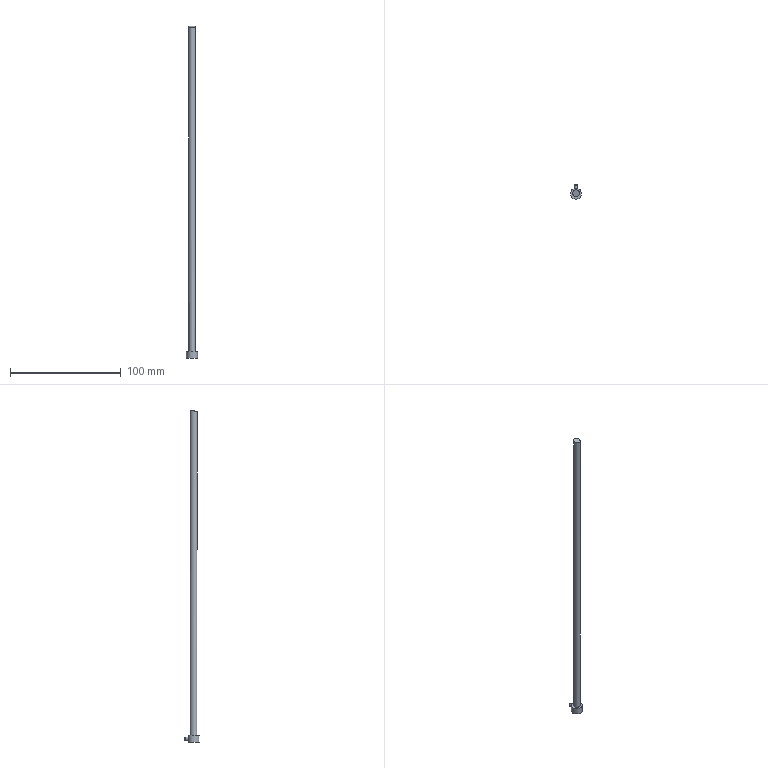Part | STEP file | E106-18-310 | 1 solid | 8 faces | box 10 x 13 x 299.38 mm | volume 8763 mm3 | cylinder 3 | plane 3 | spline 1 | cone 1 | commonest cylinder face diameters 3 x1 6 x1 10 x1